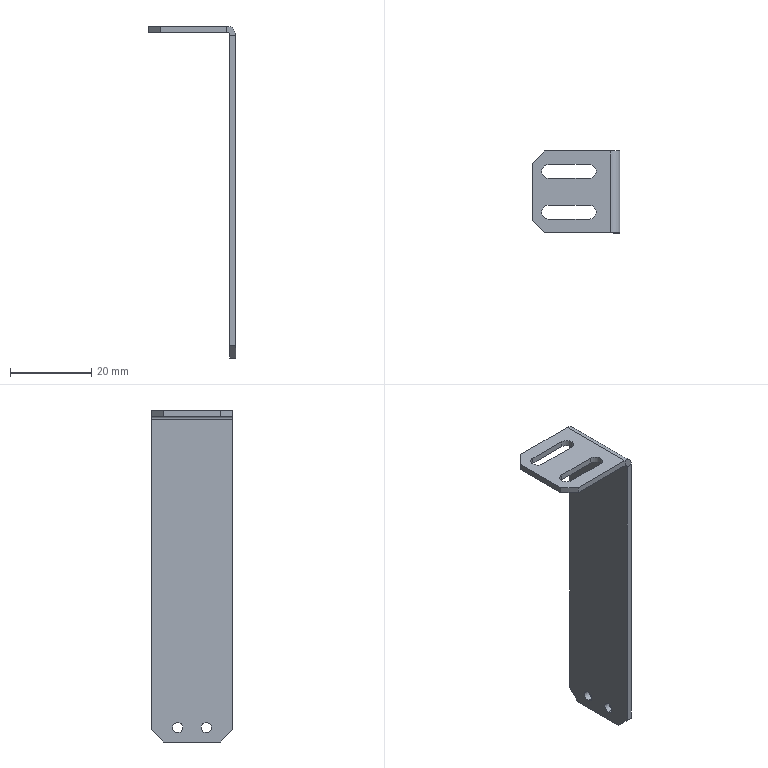Part | SolidWorks | features HoleWzd 2, Chamfer 1, FlatPattern 1, SMBaseFlange 1, SheetMetal 1 | 1 solid | 32 faces | box 21.5 x 20 x 81.5 mm | volume 2855 mm3 | plane 20 | cylinder 12 | commonest cylinder face diameters 3.4 x6 2.5 x4 1.473 x1 4.473 x1
STEP:
#1=CARTESIAN_POINT('',(-17.7,15.,1.5));
#2=VERTEX_POINT('',#1);
#3=CARTESIAN_POINT('',(-16.,16.7,1.5));
#4=VERTEX_POINT('',#3);
#5=CARTESIAN_POINT('',(-16.,15.,1.5));
#6=DIRECTION('',(0.,0.,-1.));
#7=DIRECTION('',(-1.,0.,0.));
#8=AXIS2_PLACEMENT_3D('',#5,#6,#7);
#9=CIRCLE('',#8,1.7);
#10=EDGE_CURVE('',#2,#4,#9,.T.);
#11=ORIENTED_EDGE('',*,*,#10,.F.);
#12=CARTESIAN_POINT('',(-17.7,15.,0.));
#13=VERTEX_POINT('',#12);
#14=CARTESIAN_POINT('',(-17.7,15.,0.));
#15=DIRECTION('',(0.,0.,-1.));
#16=VECTOR('',#15,1000.);
#17=LINE('',#14,#16);
#18=EDGE_CURVE('',#2,#13,#17,.T.);
#19=ORIENTED_EDGE('',*,*,#18,.T.);
#20=CARTESIAN_POINT('',(-16.,16.7,0.));
#21=VERTEX_POINT('',#20);
#22=CARTESIAN_POINT('',(-16.,15.,0.));
#23=DIRECTION('',(0.,0.,-1.));
#24=DIRECTION('',(-1.,0.,0.));
#25=AXIS2_PLACEMENT_3D('',#22,#23,#24);
#26=CIRCLE('',#25,1.7);
#27=EDGE_CURVE('',#13,#21,#26,.T.);
#28=ORIENTED_EDGE('',*,*,#27,.T.);
#29=CARTESIAN_POINT('',(-16.,16.7,0.));
#30=DIRECTION('',(0.,0.,-1.));
#31=VECTOR('',#30,1000.);
#32=LINE('',#29,#31);
#33=EDGE_CURVE('',#4,#21,#32,.T.);
#34=ORIENTED_EDGE('',*,*,#33,.F.);
#35=EDGE_LOOP('',(#11,#19,#28,#34));
#36=FACE_OUTER_BOUND('',#35,.T.);
#37=CARTESIAN_POINT('',(-16.,15.,0.));
#38=DIRECTION('',(0.,0.,-1.));
#39=DIRECTION('',(-1.,0.,0.));
#40=AXIS2_PLACEMENT_3D('',#37,#38,#39);
#41=CYLINDRICAL_SURFACE('',#40,1.7);
#42=ADVANCED_FACE('',(#36),#41,.F.);
#43=CARTESIAN_POINT('',(-17.7,5.,1.5));
#44=VERTEX_POINT('',#43);
#45=CARTESIAN_POINT('',(-16.,6.7,1.5));
#46=VERTEX_POINT('',#45);
#47=CARTESIAN_POINT('',(-16.,5.,1.5));
#48=DIRECTION('',(0.,0.,-1.));
#49=DIRECTION('',(-1.,0.,0.));
#50=AXIS2_PLACEMENT_3D('',#47,#48,#49);
#51=CIRCLE('',#50,1.7);
#52=EDGE_CURVE('',#44,#46,#51,.T.);
#53=ORIENTED_EDGE('',*,*,#52,.F.);
#54=CARTESIAN_POINT('',(-17.7,5.,0.));
#55=VERTEX_POINT('',#54);
#56=CARTESIAN_POINT('',(-17.7,5.,0.));
#57=DIRECTION('',(0.,0.,-1.));
#58=VECTOR('',#57,1000.);
#59=LINE('',#56,#58);
#60=EDGE_CURVE('',#44,#55,#59,.T.);
#61=ORIENTED_EDGE('',*,*,#60,.T.);
#62=CARTESIAN_POINT('',(-16.,6.7,0.));
#63=VERTEX_POINT('',#62);
#64=CARTESIAN_POINT('',(-16.,5.,0.));
#65=DIRECTION('',(0.,0.,-1.));
#66=DIRECTION('',(-1.,0.,0.));
#67=AXIS2_PLACEMENT_3D('',#64,#65,#66);
#68=CIRCLE('',#67,1.7);
#69=EDGE_CURVE('',#55,#63,#68,.T.);
#70=ORIENTED_EDGE('',*,*,#69,.T.);
#71=CARTESIAN_POINT('',(-16.,6.7,0.));
#72=DIRECTION('',(0.,0.,-1.));
#73=VECTOR('',#72,1000.);
#74=LINE('',#71,#73);
#75=EDGE_CURVE('',#46,#63,#74,.T.);
#76=ORIENTED_EDGE('',*,*,#75,.F.);
#77=EDGE_LOOP('',(#53,#61,#70,#76));
#78=FACE_OUTER_BOUND('',#77,.T.);
#79=CARTESIAN_POINT('',(-16.,5.,0.));
#80=DIRECTION('',(0.,0.,-1.));
#81=DIRECTION('',(-1.,0.,0.));
#82=AXIS2_PLACEMENT_3D('',#79,#80,#81);
#83=CYLINDRICAL_SURFACE('',#82,1.7);
#84=ADVANCED_FACE('',(#78),#83,.F.);
#85=CARTESIAN_POINT('',(0.,13.5,-77.75));
#86=VERTEX_POINT('',#85);
#87=CARTESIAN_POINT('',(0.,13.5,-75.25));
#88=VERTEX_POINT('',#87);
#89=CARTESIAN_POINT('',(0.,13.5,-76.5));
#90=DIRECTION('',(-1.,0.,0.));
#91=DIRECTION('',(0.,0.,1.));
#92=AXIS2_PLACEMENT_3D('',#89,#90,#91);
#93=CIRCLE('',#92,1.25);
#94=EDGE_CURVE('',#86,#88,#93,.T.);
#95=ORIENTED_EDGE('',*,*,#94,.T.);
#96=CARTESIAN_POINT('',(1.5,13.5,-75.25));
#97=VERTEX_POINT('',#96);
#98=CARTESIAN_POINT('',(1.5,13.5,-75.25));
#99=DIRECTION('',(1.,0.,0.));
#100=VECTOR('',#99,1000.);
#101=LINE('',#98,#100);
#102=EDGE_CURVE('',#88,#97,#101,.T.);
#103=ORIENTED_EDGE('',*,*,#102,.T.);
#104=CARTESIAN_POINT('',(1.5,13.5,-77.75));
#105=VERTEX_POINT('',#104);
#106=CARTESIAN_POINT('',(1.5,13.5,-76.5));
#107=DIRECTION('',(1.,0.,0.));
#108=DIRECTION('',(0.,0.,-1.));
#109=AXIS2_PLACEMENT_3D('',#106,#107,#108);
#110=CIRCLE('',#109,1.25);
#111=EDGE_CURVE('',#97,#105,#110,.T.);
#112=ORIENTED_EDGE('',*,*,#111,.T.);
#113=CARTESIAN_POINT('',(1.5,13.5,-77.75));
#114=DIRECTION('',(1.,0.,0.));
#115=VECTOR('',#114,1000.);
#116=LINE('',#113,#115);
#117=EDGE_CURVE('',#86,#105,#116,.T.);
#118=ORIENTED_EDGE('',*,*,#117,.F.);
#119=EDGE_LOOP('',(#95,#103,#112,#118));
#120=FACE_OUTER_BOUND('',#119,.T.);
#121=CARTESIAN_POINT('',(1.5,13.5,-76.5));
#122=DIRECTION('',(1.,0.,0.));
#123=DIRECTION('',(0.,0.,-1.));
#124=AXIS2_PLACEMENT_3D('',#121,#122,#123);
#125=CYLINDRICAL_SURFACE('',#124,1.25);
#126=ADVANCED_FACE('',(#120),#125,.F.);
#127=CARTESIAN_POINT('',(0.,6.5,-77.75));
#128=VERTEX_POINT('',#127);
#129=CARTESIAN_POINT('',(0.,6.5,-75.25));
#130=VERTEX_POINT('',#129);
#131=CARTESIAN_POINT('',(0.,6.5,-76.5));
#132=DIRECTION('',(-1.,0.,0.));
#133=DIRECTION('',(0.,0.,1.));
#134=AXIS2_PLACEMENT_3D('',#131,#132,#133);
#135=CIRCLE('',#134,1.25);
#136=EDGE_CURVE('',#128,#130,#135,.T.);
#137=ORIENTED_EDGE('',*,*,#136,.T.);
#138=CARTESIAN_POINT('',(1.5,6.5,-75.25));
#139=VERTEX_POINT('',#138);
#140=CARTESIAN_POINT('',(1.5,6.5,-75.25));
#141=DIRECTION('',(1.,0.,0.));
#142=VECTOR('',#141,1000.);
#143=LINE('',#140,#142);
#144=EDGE_CURVE('',#130,#139,#143,.T.);
#145=ORIENTED_EDGE('',*,*,#144,.T.);
#146=CARTESIAN_POINT('',(1.5,6.5,-77.75));
#147=VERTEX_POINT('',#146);
#148=CARTESIAN_POINT('',(1.5,6.5,-76.5));
#149=DIRECTION('',(1.,0.,0.));
#150=DIRECTION('',(0.,0.,-1.));
#151=AXIS2_PLACEMENT_3D('',#148,#149,#150);
#152=CIRCLE('',#151,1.25);
#153=EDGE_CURVE('',#139,#147,#152,.T.);
#154=ORIENTED_EDGE('',*,*,#153,.T.);
#155=CARTESIAN_POINT('',(1.5,6.5,-77.75));
#156=DIRECTION('',(1.,0.,0.));
#157=VECTOR('',#156,1000.);
#158=LINE('',#155,#157);
#159=EDGE_CURVE('',#128,#147,#158,.T.);
#160=ORIENTED_EDGE('',*,*,#159,.F.);
#161=EDGE_LOOP('',(#137,#145,#154,#160));
#162=FACE_OUTER_BOUND('',#161,.T.);
#163=CARTESIAN_POINT('',(1.5,6.5,-76.5));
#164=DIRECTION('',(1.,0.,0.));
#165=DIRECTION('',(0.,0.,-1.));
#166=AXIS2_PLACEMENT_3D('',#163,#164,#165);
#167=CYLINDRICAL_SURFACE('',#166,1.25);
#168=ADVANCED_FACE('',(#162),#167,.F.);
#169=CARTESIAN_POINT('',(0.,20.,-0.7366));
#170=VERTEX_POINT('',#169);
#171=CARTESIAN_POINT('',(1.5,20.,-0.7366));
#172=VERTEX_POINT('',#171);
#173=CARTESIAN_POINT('',(0.,20.,-0.7366));
#174=DIRECTION('',(1.,0.,0.));
#175=VECTOR('',#174,1000.);
#176=LINE('',#173,#175);
#177=EDGE_CURVE('',#170,#172,#176,.T.);
#178=ORIENTED_EDGE('',*,*,#177,.F.);
#179=CARTESIAN_POINT('',(-0.7366,20.,0.));
#180=VERTEX_POINT('',#179);
#181=CARTESIAN_POINT('',(-0.7366,20.,-0.7366));
#182=DIRECTION('',(0.,1.,0.));
#183=DIRECTION('',(0.,0.,-1.));
#184=AXIS2_PLACEMENT_3D('',#181,#182,#183);
#185=CIRCLE('',#184,0.7366);
#186=EDGE_CURVE('',#180,#170,#185,.T.);
#187=ORIENTED_EDGE('',*,*,#186,.F.);
#188=CARTESIAN_POINT('',(-0.7366,20.,1.5));
#189=VERTEX_POINT('',#188);
#190=CARTESIAN_POINT('',(-0.7366,20.,1.5));
#191=DIRECTION('',(0.,0.,-1.));
#192=VECTOR('',#191,1000.);
#193=LINE('',#190,#192);
#194=EDGE_CURVE('',#189,#180,#193,.T.);
#195=ORIENTED_EDGE('',*,*,#194,.F.);
#196=CARTESIAN_POINT('',(-0.7366,20.,-0.7366));
#197=DIRECTION('',(0.,1.,0.));
#198=DIRECTION('',(1.,0.,0.));
#199=AXIS2_PLACEMENT_3D('',#196,#197,#198);
#200=CIRCLE('',#199,2.237);
#201=EDGE_CURVE('',#189,#172,#200,.T.);
#202=ORIENTED_EDGE('',*,*,#201,.T.);
#203=EDGE_LOOP('',(#178,#187,#195,#202));
#204=FACE_OUTER_BOUND('',#203,.T.);
#205=CARTESIAN_POINT('',(0.,20.,-0.7366));
#206=DIRECTION('',(0.,1.,0.));
#207=DIRECTION('',(0.,0.,1.));
#208=AXIS2_PLACEMENT_3D('',#205,#206,#207);
#209=PLANE('',#208);
#210=ADVANCED_FACE('',(#204),#209,.T.);
#211=CARTESIAN_POINT('',(1.5,20.,-77.));
#212=VERTEX_POINT('',#211);
#213=CARTESIAN_POINT('',(1.5,20.,0.));
#214=DIRECTION('',(0.,0.,-1.));
#215=VECTOR('',#214,1000.);
#216=LINE('',#213,#215);
#217=EDGE_CURVE('',#172,#212,#216,.T.);
#218=ORIENTED_EDGE('',*,*,#217,.T.);
#219=CARTESIAN_POINT('',(0.,20.,-77.));
#220=VERTEX_POINT('',#219);
#221=CARTESIAN_POINT('',(-0.7366,20.,-77.));
#222=DIRECTION('',(-1.,0.,0.));
#223=VECTOR('',#222,1000.);
#224=LINE('',#221,#223);
#225=EDGE_CURVE('',#212,#220,#224,.T.);
#226=ORIENTED_EDGE('',*,*,#225,.T.);
#227=CARTESIAN_POINT('',(0.,20.,0.));
#228=DIRECTION('',(0.,0.,-1.));
#229=VECTOR('',#228,1000.);
#230=LINE('',#227,#229);
#231=EDGE_CURVE('',#170,#220,#230,.T.);
#232=ORIENTED_EDGE('',*,*,#231,.F.);
#233=ORIENTED_EDGE('',*,*,#177,.T.);
#234=EDGE_LOOP('',(#218,#226,#232,#233));
#235=FACE_OUTER_BOUND('',#234,.T.);
#236=CARTESIAN_POINT('',(-0.7366,20.,1.5));
#237=DIRECTION('',(0.,1.,0.));
#238=DIRECTION('',(0.,0.,1.));
#239=AXIS2_PLACEMENT_3D('',#236,#237,#238);
#240=PLANE('',#239);
#241=ADVANCED_FACE('',(#235),#240,.T.);
#242=CARTESIAN_POINT('',(-0.7366,0.,0.));
#243=VERTEX_POINT('',#242);
#244=CARTESIAN_POINT('',(-0.7366,0.,1.5));
#245=VERTEX_POINT('',#244);
#246=CARTESIAN_POINT('',(-0.7366,0.,0.));
#247=DIRECTION('',(0.,0.,1.));
#248=VECTOR('',#247,1000.);
#249=LINE('',#246,#248);
#250=EDGE_CURVE('',#243,#245,#249,.T.);
#251=ORIENTED_EDGE('',*,*,#250,.F.);
#252=CARTESIAN_POINT('',(0.,0.,-0.7366));
#253=VERTEX_POINT('',#252);
#254=CARTESIAN_POINT('',(-0.7366,0.,-0.7366));
#255=DIRECTION('',(0.,1.,0.));
#256=DIRECTION('',(0.,0.,-1.));
#257=AXIS2_PLACEMENT_3D('',#254,#255,#256);
#258=CIRCLE('',#257,0.7366);
#259=EDGE_CURVE('',#243,#253,#258,.T.);
#260=ORIENTED_EDGE('',*,*,#259,.T.);
#261=CARTESIAN_POINT('',(1.5,0.,-0.7366));
#262=VERTEX_POINT('',#261);
#263=CARTESIAN_POINT('',(1.5,0.,-0.7366));
#264=DIRECTION('',(-1.,0.,0.));
#265=VECTOR('',#264,1000.);
#266=LINE('',#263,#265);
#267=EDGE_CURVE('',#262,#253,#266,.T.);
#268=ORIENTED_EDGE('',*,*,#267,.F.);
#269=CARTESIAN_POINT('',(-0.7366,0.,-0.7366));
#270=DIRECTION('',(0.,1.,0.));
#271=DIRECTION('',(1.,0.,0.));
#272=AXIS2_PLACEMENT_3D('',#269,#270,#271);
#273=CIRCLE('',#272,2.237);
#274=EDGE_CURVE('',#245,#262,#273,.T.);
#275=ORIENTED_EDGE('',*,*,#274,.F.);
#276=EDGE_LOOP('',(#251,#260,#268,#275));
#277=FACE_OUTER_BOUND('',#276,.T.);
#278=CARTESIAN_POINT('',(-0.7366,0.,0.));
#279=DIRECTION('',(0.,-1.,0.));
#280=DIRECTION('',(0.,0.,-1.));
#281=AXIS2_PLACEMENT_3D('',#278,#279,#280);
#282=PLANE('',#281);
#283=ADVANCED_FACE('',(#277),#282,.T.);
#284=CARTESIAN_POINT('',(-17.,0.,1.5));
#285=VERTEX_POINT('',#284);
#286=CARTESIAN_POINT('',(-20.,0.,1.5));
#287=DIRECTION('',(1.,0.,0.));
#288=VECTOR('',#287,1000.);
#289=LINE('',#286,#288);
#290=EDGE_CURVE('',#285,#245,#289,.T.);
#291=ORIENTED_EDGE('',*,*,#290,.F.);
#292=CARTESIAN_POINT('',(-17.,0.,0.));
#293=VERTEX_POINT('',#292);
#294=CARTESIAN_POINT('',(-17.,0.,-0.7366));
#295=DIRECTION('',(0.,0.,-1.));
#296=VECTOR('',#295,1000.);
#297=LINE('',#294,#296);
#298=EDGE_CURVE('',#285,#293,#297,.T.);
#299=ORIENTED_EDGE('',*,*,#298,.T.);
#300=CARTESIAN_POINT('',(-20.,0.,0.));
#301=DIRECTION('',(1.,0.,0.));
#302=VECTOR('',#301,1000.);
#303=LINE('',#300,#302);
#304=EDGE_CURVE('',#293,#243,#303,.T.);
#305=ORIENTED_EDGE('',*,*,#304,.T.);
#306=ORIENTED_EDGE('',*,*,#250,.T.);
#307=EDGE_LOOP('',(#291,#299,#305,#306));
#308=FACE_OUTER_BOUND('',#307,.T.);
#309=CARTESIAN_POINT('',(1.5,0.,-0.7366));
#310=DIRECTION('',(0.,-1.,0.));
#311=DIRECTION('',(0.,0.,-1.));
#312=AXIS2_PLACEMENT_3D('',#309,#310,#311);
#313=PLANE('',#312);
#314=ADVANCED_FACE('',(#308),#313,.T.);
#315=CARTESIAN_POINT('',(1.5,13.5,-76.5));
#316=DIRECTION('',(1.,0.,0.));
#317=DIRECTION('',(0.,0.,-1.));
#318=AXIS2_PLACEMENT_3D('',#315,#316,#317);
#319=CIRCLE('',#318,1.25);
#320=EDGE_CURVE('',#105,#97,#319,.T.);
#321=ORIENTED_EDGE('',*,*,#320,.F.);
#322=ORIENTED_EDGE('',*,*,#111,.F.);
#323=EDGE_LOOP('',(#321,#322));
#324=FACE_BOUND('',#323,.T.);
#325=CARTESIAN_POINT('',(1.5,6.5,-76.5));
#326=DIRECTION('',(1.,0.,0.));
#327=DIRECTION('',(0.,0.,-1.));
#328=AXIS2_PLACEMENT_3D('',#325,#326,#327);
#329=CIRCLE('',#328,1.25);
#330=EDGE_CURVE('',#147,#139,#329,.T.);
#331=ORIENTED_EDGE('',*,*,#330,.F.);
#332=ORIENTED_EDGE('',*,*,#153,.F.);
#333=EDGE_LOOP('',(#331,#332));
#334=FACE_BOUND('',#333,.T.);
#335=CARTESIAN_POINT('',(1.5,0.,-77.));
#336=VERTEX_POINT('',#335);
#337=CARTESIAN_POINT('',(1.5,0.,0.));
#338=DIRECTION('',(0.,0.,-1.));
#339=VECTOR('',#338,1000.);
#340=LINE('',#337,#339);
#341=EDGE_CURVE('',#262,#336,#340,.T.);
#342=ORIENTED_EDGE('',*,*,#341,.T.);
#343=CARTESIAN_POINT('',(1.5,3.,-80.));
#344=VERTEX_POINT('',#343);
#345=CARTESIAN_POINT('',(1.5,0.,-77.));
#346=DIRECTION('',(0.,0.7071,-0.7071));
#347=VECTOR('',#346,1000.);
#348=LINE('',#345,#347);
#349=EDGE_CURVE('',#336,#344,#348,.T.);
#350=ORIENTED_EDGE('',*,*,#349,.T.);
#351=CARTESIAN_POINT('',(1.5,17.,-80.));
#352=VERTEX_POINT('',#351);
#353=CARTESIAN_POINT('',(1.5,20.,-80.));
#354=DIRECTION('',(0.,-1.,0.));
#355=VECTOR('',#354,1000.);
#356=LINE('',#353,#355);
#357=EDGE_CURVE('',#352,#344,#356,.T.);
#358=ORIENTED_EDGE('',*,*,#357,.F.);
#359=CARTESIAN_POINT('',(1.5,17.,-80.));
#360=DIRECTION('',(0.,0.7071,0.7071));
#361=VECTOR('',#360,1000.);
#362=LINE('',#359,#361);
#363=EDGE_CURVE('',#352,#212,#362,.T.);
#364=ORIENTED_EDGE('',*,*,#363,.T.);
#365=ORIENTED_EDGE('',*,*,#217,.F.);
#366=CARTESIAN_POINT('',(1.5,20.,-0.7366));
#367=DIRECTION('',(0.,-1.,0.));
#368=VECTOR('',#367,1000.);
#369=LINE('',#366,#368);
#370=EDGE_CURVE('',#172,#262,#369,.T.);
#371=ORIENTED_EDGE('',*,*,#370,.T.);
#372=EDGE_LOOP('',(#342,#350,#358,#364,#365,#371));
#373=FACE_OUTER_BOUND('',#372,.T.);
#374=CARTESIAN_POINT('',(1.5,20.,0.));
#375=DIRECTION('',(-1.,0.,0.));
#376=DIRECTION('',(0.,0.,1.));
#377=AXIS2_PLACEMENT_3D('',#374,#375,#376);
#378=PLANE('',#377);
#379=ADVANCED_FACE('',(#324,#334,#373),#378,.F.);
#380=ORIENTED_EDGE('',*,*,#357,.T.);
#381=CARTESIAN_POINT('',(0.,3.,-80.));
#382=VERTEX_POINT('',#381);
#383=CARTESIAN_POINT('',(0.,3.,-80.));
#384=DIRECTION('',(-1.,0.,0.));
#385=VECTOR('',#384,1000.);
#386=LINE('',#383,#385);
#387=EDGE_CURVE('',#344,#382,#386,.T.);
#388=ORIENTED_EDGE('',*,*,#387,.T.);
#389=CARTESIAN_POINT('',(0.,17.,-80.));
#390=VERTEX_POINT('',#389);
#391=CARTESIAN_POINT('',(0.,20.,-80.));
#392=DIRECTION('',(0.,-1.,0.));
#393=VECTOR('',#392,1000.);
#394=LINE('',#391,#393);
#395=EDGE_CURVE('',#390,#382,#394,.T.);
#396=ORIENTED_EDGE('',*,*,#395,.F.);
#397=CARTESIAN_POINT('',(0.,17.,-80.));
#398=DIRECTION('',(1.,0.,0.));
#399=VECTOR('',#398,1000.);
#400=LINE('',#397,#399);
#401=EDGE_CURVE('',#390,#352,#400,.T.);
#402=ORIENTED_EDGE('',*,*,#401,.T.);
#403=EDGE_LOOP('',(#380,#388,#396,#402));
#404=FACE_OUTER_BOUND('',#403,.T.);
#405=CARTESIAN_POINT('',(0.,20.,-80.));
#406=DIRECTION('',(0.,0.,-1.));
#407=DIRECTION('',(-1.,0.,0.));
#408=AXIS2_PLACEMENT_3D('',#405,#406,#407);
#409=PLANE('',#408);
#410=ADVANCED_FACE('',(#404),#409,.T.);
#411=ORIENTED_EDGE('',*,*,#94,.F.);
#412=CARTESIAN_POINT('',(0.,13.5,-76.5));
#413=DIRECTION('',(-1.,0.,0.));
#414=DIRECTION('',(0.,0.,1.));
#415=AXIS2_PLACEMENT_3D('',#412,#413,#414);
#416=CIRCLE('',#415,1.25);
#417=EDGE_CURVE('',#88,#86,#416,.T.);
#418=ORIENTED_EDGE('',*,*,#417,.F.);
#419=EDGE_LOOP('',(#411,#418));
#420=FACE_BOUND('',#419,.T.);
#421=ORIENTED_EDGE('',*,*,#136,.F.);
#422=CARTESIAN_POINT('',(0.,6.5,-76.5));
#423=DIRECTION('',(-1.,0.,0.));
#424=DIRECTION('',(0.,0.,1.));
#425=AXIS2_PLACEMENT_3D('',#422,#423,#424);
#426=CIRCLE('',#425,1.25);
#427=EDGE_CURVE('',#130,#128,#426,.T.);
#428=ORIENTED_EDGE('',*,*,#427,.F.);
#429=EDGE_LOOP('',(#421,#428));
#430=FACE_BOUND('',#429,.T.);
#431=ORIENTED_EDGE('',*,*,#395,.T.);
#432=CARTESIAN_POINT('',(0.,0.,-77.));
#433=VERTEX_POINT('',#432);
#434=CARTESIAN_POINT('',(0.,-28.5,-48.5));
#435=DIRECTION('',(0.,-0.7071,0.7071));
#436=VECTOR('',#435,1000.);
#437=LINE('',#434,#436);
#438=EDGE_CURVE('',#382,#433,#437,.T.);
#439=ORIENTED_EDGE('',*,*,#438,.T.);
#440=CARTESIAN_POINT('',(0.,0.,0.));
#441=DIRECTION('',(0.,0.,-1.));
#442=VECTOR('',#441,1000.);
#443=LINE('',#440,#442);
#444=EDGE_CURVE('',#253,#433,#443,.T.);
#445=ORIENTED_EDGE('',*,*,#444,.F.);
#446=CARTESIAN_POINT('',(0.,20.,-0.7366));
#447=DIRECTION('',(0.,-1.,0.));
#448=VECTOR('',#447,1000.);
#449=LINE('',#446,#448);
#450=EDGE_CURVE('',#170,#253,#449,.T.);
#451=ORIENTED_EDGE('',*,*,#450,.F.);
#452=ORIENTED_EDGE('',*,*,#231,.T.);
#453=CARTESIAN_POINT('',(0.,58.5,-38.5));
#454=DIRECTION('',(0.,-0.7071,-0.7071));
#455=VECTOR('',#454,1000.);
#456=LINE('',#453,#455);
#457=EDGE_CURVE('',#220,#390,#456,.T.);
#458=ORIENTED_EDGE('',*,*,#457,.T.);
#459=EDGE_LOOP('',(#431,#439,#445,#451,#452,#458));
#460=FACE_OUTER_BOUND('',#459,.T.);
#461=CARTESIAN_POINT('',(0.,20.,0.));
#462=DIRECTION('',(-1.,0.,0.));
#463=DIRECTION('',(0.,0.,1.));
#464=AXIS2_PLACEMENT_3D('',#461,#462,#463);
#465=PLANE('',#464);
#466=ADVANCED_FACE('',(#420,#430,#460),#465,.T.);
#467=ORIENTED_EDGE('',*,*,#259,.F.);
#468=CARTESIAN_POINT('',(-0.7366,20.,0.));
#469=DIRECTION('',(0.,-1.,0.));
#470=VECTOR('',#469,1000.);
#471=LINE('',#468,#470);
#472=EDGE_CURVE('',#180,#243,#471,.T.);
#473=ORIENTED_EDGE('',*,*,#472,.F.);
#474=ORIENTED_EDGE('',*,*,#186,.T.);
#475=ORIENTED_EDGE('',*,*,#450,.T.);
#476=EDGE_LOOP('',(#467,#473,#474,#475));
#477=FACE_OUTER_BOUND('',#476,.T.);
#478=CARTESIAN_POINT('',(-0.7366,20.,-0.7366));
#479=DIRECTION('',(0.,-1.,0.));
#480=DIRECTION('',(0.,0.,-1.));
#481=AXIS2_PLACEMENT_3D('',#478,#479,#480);
#482=CYLINDRICAL_SURFACE('',#481,0.7366);
#483=ADVANCED_FACE('',(#477),#482,.F.);
#484=CARTESIAN_POINT('',(-6.,16.7,0.));
#485=VERTEX_POINT('',#484);
#486=CARTESIAN_POINT('',(-6.,13.3,0.));
#487=VERTEX_POINT('',#486);
#488=CARTESIAN_POINT('',(-6.,15.,0.));
#489=DIRECTION('',(0.,0.,-1.));
#490=DIRECTION('',(-1.,0.,0.));
#491=AXIS2_PLACEMENT_3D('',#488,#489,#490);
#492=CIRCLE('',#491,1.7);
#493=EDGE_CURVE('',#485,#487,#492,.T.);
#494=ORIENTED_EDGE('',*,*,#493,.F.);
#495=CARTESIAN_POINT('',(-16.,16.7,0.));
#496=DIRECTION('',(1.,0.,0.));
#497=VECTOR('',#496,1000.);
#498=LINE('',#495,#497);
#499=EDGE_CURVE('',#21,#485,#498,.T.);
#500=ORIENTED_EDGE('',*,*,#499,.F.);
#501=ORIENTED_EDGE('',*,*,#27,.F.);
#502=CARTESIAN_POINT('',(-16.,13.3,0.));
#503=VERTEX_POINT('',#502);
#504=CARTESIAN_POINT('',(-16.,15.,0.));
#505=DIRECTION('',(0.,0.,-1.));
#506=DIRECTION('',(-1.,0.,0.));
#507=AXIS2_PLACEMENT_3D('',#504,#505,#506);
#508=CIRCLE('',#507,1.7);
#509=EDGE_CURVE('',#503,#13,#508,.T.);
#510=ORIENTED_EDGE('',*,*,#509,.F.);
#511=CARTESIAN_POINT('',(-16.,13.3,0.));
#512=DIRECTION('',(1.,0.,0.));
#513=VECTOR('',#512,1000.);
#514=LINE('',#511,#513);
#515=EDGE_CURVE('',#503,#487,#514,.T.);
#516=ORIENTED_EDGE('',*,*,#515,.T.);
#517=EDGE_LOOP('',(#494,#500,#501,#510,#516));
#518=FACE_BOUND('',#517,.T.);
#519=CARTESIAN_POINT('',(-6.,6.7,0.));
#520=VERTEX_POINT('',#519);
#521=CARTESIAN_POINT('',(-16.,6.7,0.));
#522=DIRECTION('',(1.,0.,0.));
#523=VECTOR('',#522,1000.);
#524=LINE('',#521,#523);
#525=EDGE_CURVE('',#63,#520,#524,.T.);
#526=ORIENTED_EDGE('',*,*,#525,.F.);
#527=ORIENTED_EDGE('',*,*,#69,.F.);
#528=CARTESIAN_POINT('',(-16.,3.3,0.));
#529=VERTEX_POINT('',#528);
#530=CARTESIAN_POINT('',(-16.,5.,0.));
#531=DIRECTION('',(0.,0.,-1.));
#532=DIRECTION('',(-1.,0.,0.));
#533=AXIS2_PLACEMENT_3D('',#530,#531,#532);
#534=CIRCLE('',#533,1.7);
#535=EDGE_CURVE('',#529,#55,#534,.T.);
#536=ORIENTED_EDGE('',*,*,#535,.F.);
#537=CARTESIAN_POINT('',(-6.,3.3,0.));
#538=VERTEX_POINT('',#537);
#539=CARTESIAN_POINT('',(-16.,3.3,0.));
#540=DIRECTION('',(1.,0.,0.));
#541=VECTOR('',#540,1000.);
#542=LINE('',#539,#541);
#543=EDGE_CURVE('',#529,#538,#542,.T.);
#544=ORIENTED_EDGE('',*,*,#543,.T.);
#545=CARTESIAN_POINT('',(-6.,5.,0.));
#546=DIRECTION('',(0.,0.,-1.));
#547=DIRECTION('',(-1.,0.,0.));
#548=AXIS2_PLACEMENT_3D('',#545,#546,#547);
#549=CIRCLE('',#548,1.7);
#550=EDGE_CURVE('',#520,#538,#549,.T.);
#551=ORIENTED_EDGE('',*,*,#550,.F.);
#552=EDGE_LOOP('',(#526,#527,#536,#544,#551));
#553=FACE_BOUND('',#552,.T.);
#554=CARTESIAN_POINT('',(-20.,17.,0.));
#555=VERTEX_POINT('',#554);
#556=CARTESIAN_POINT('',(-20.,3.,0.));
#557=VERTEX_POINT('',#556);
#558=CARTESIAN_POINT('',(-20.,20.,0.));
#559=DIRECTION('',(0.,-1.,0.));
#560=VECTOR('',#559,1000.);
#561=LINE('',#558,#560);
#562=EDGE_CURVE('',#555,#557,#561,.T.);
#563=ORIENTED_EDGE('',*,*,#562,.F.);
#564=CARTESIAN_POINT('',(-17.,20.,0.));
#565=VERTEX_POINT('',#564);
#566=CARTESIAN_POINT('',(-18.5,18.5,0.));
#567=DIRECTION('',(0.7071,0.7071,0.));
#568=VECTOR('',#567,1000.);
#569=LINE('',#566,#568);
#570=EDGE_CURVE('',#555,#565,#569,.T.);
#571=ORIENTED_EDGE('',*,*,#570,.T.);
#572=CARTESIAN_POINT('',(-20.,20.,0.));
#573=DIRECTION('',(1.,0.,0.));
#574=VECTOR('',#573,1000.);
#575=LINE('',#572,#574);
#576=EDGE_CURVE('',#565,#180,#575,.T.);
#577=ORIENTED_EDGE('',*,*,#576,.T.);
#578=ORIENTED_EDGE('',*,*,#472,.T.);
#579=ORIENTED_EDGE('',*,*,#304,.F.);
#580=CARTESIAN_POINT('',(-28.5,11.5,0.));
#581=DIRECTION('',(-0.7071,0.7071,0.));
#582=VECTOR('',#581,1000.);
#583=LINE('',#580,#582);
#584=EDGE_CURVE('',#293,#557,#583,.T.);
#585=ORIENTED_EDGE('',*,*,#584,.T.);
#586=EDGE_LOOP('',(#563,#571,#577,#578,#579,#585));
#587=FACE_OUTER_BOUND('',#586,.T.);
#588=CARTESIAN_POINT('',(-20.,20.,0.));
#589=DIRECTION('',(0.,0.,-1.));
#590=DIRECTION('',(-1.,0.,0.));
#591=AXIS2_PLACEMENT_3D('',#588,#589,#590);
#592=PLANE('',#591);
#593=ADVANCED_FACE('',(#518,#553,#587),#592,.T.);
#594=CARTESIAN_POINT('',(-20.,17.,1.5));
#595=VERTEX_POINT('',#594);
#596=CARTESIAN_POINT('',(-20.,3.,1.5));
#597=VERTEX_POINT('',#596);
#598=CARTESIAN_POINT('',(-20.,20.,1.5));
#599=DIRECTION('',(0.,-1.,0.));
#600=VECTOR('',#599,1000.);
#601=LINE('',#598,#600);
#602=EDGE_CURVE('',#595,#597,#601,.T.);
#603=ORIENTED_EDGE('',*,*,#602,.F.);
#604=CARTESIAN_POINT('',(-20.,17.,0.));
#605=DIRECTION('',(0.,0.,-1.));
#606=VECTOR('',#605,1000.);
#607=LINE('',#604,#606);
#608=EDGE_CURVE('',#595,#555,#607,.T.);
#609=ORIENTED_EDGE('',*,*,#608,.T.);
#610=ORIENTED_EDGE('',*,*,#562,.T.);
#611=CARTESIAN_POINT('',(-20.,3.,1.5));
#612=DIRECTION('',(0.,0.,1.));
#613=VECTOR('',#612,1000.);
#614=LINE('',#611,#613);
#615=EDGE_CURVE('',#557,#597,#614,.T.);
#616=ORIENTED_EDGE('',*,*,#615,.T.);
#617=EDGE_LOOP('',(#603,#609,#610,#616));
#618=FACE_OUTER_BOUND('',#617,.T.);
#619=CARTESIAN_POINT('',(-20.,20.,1.5));
#620=DIRECTION('',(-1.,0.,0.));
#621=DIRECTION('',(0.,0.,1.));
#622=AXIS2_PLACEMENT_3D('',#619,#620,#621);
#623=PLANE('',#622);
#624=ADVANCED_FACE('',(#618),#623,.T.);
#625=CARTESIAN_POINT('',(-6.,16.7,1.5));
#626=VERTEX_POINT('',#625);
#627=CARTESIAN_POINT('',(-6.,13.3,1.5));
#628=VERTEX_POINT('',#627);
#629=CARTESIAN_POINT('',(-6.,15.,1.5));
#630=DIRECTION('',(0.,0.,-1.));
#631=DIRECTION('',(-1.,0.,0.));
#632=AXIS2_PLACEMENT_3D('',#629,#630,#631);
#633=CIRCLE('',#632,1.7);
#634=EDGE_CURVE('',#626,#628,#633,.T.);
#635=ORIENTED_EDGE('',*,*,#634,.T.);
#636=CARTESIAN_POINT('',(-16.,13.3,1.5));
#637=VERTEX_POINT('',#636);
#638=CARTESIAN_POINT('',(-20.,13.3,1.5));
#639=DIRECTION('',(-1.,0.,0.));
#640=VECTOR('',#639,1000.);
#641=LINE('',#638,#640);
#642=EDGE_CURVE('',#628,#637,#641,.T.);
#643=ORIENTED_EDGE('',*,*,#642,.T.);
#644=CARTESIAN_POINT('',(-16.,15.,1.5));
#645=DIRECTION('',(0.,0.,-1.));
#646=DIRECTION('',(-1.,0.,0.));
#647=AXIS2_PLACEMENT_3D('',#644,#645,#646);
#648=CIRCLE('',#647,1.7);
#649=EDGE_CURVE('',#637,#2,#648,.T.);
#650=ORIENTED_EDGE('',*,*,#649,.T.);
#651=ORIENTED_EDGE('',*,*,#10,.T.);
#652=CARTESIAN_POINT('',(-20.,16.7,1.5));
#653=DIRECTION('',(1.,0.,0.));
#654=VECTOR('',#653,1000.);
#655=LINE('',#652,#654);
#656=EDGE_CURVE('',#4,#626,#655,.T.);
#657=ORIENTED_EDGE('',*,*,#656,.T.);
#658=EDGE_LOOP('',(#635,#643,#650,#651,#657));
#659=FACE_BOUND('',#658,.T.);
#660=CARTESIAN_POINT('',(-6.,6.7,1.5));
#661=VERTEX_POINT('',#660);
#662=CARTESIAN_POINT('',(-6.,3.3,1.5));
#663=VERTEX_POINT('',#662);
#664=CARTESIAN_POINT('',(-6.,5.,1.5));
#665=DIRECTION('',(0.,0.,-1.));
#666=DIRECTION('',(-1.,0.,0.));
#667=AXIS2_PLACEMENT_3D('',#664,#665,#666);
#668=CIRCLE('',#667,1.7);
#669=EDGE_CURVE('',#661,#663,#668,.T.);
#670=ORIENTED_EDGE('',*,*,#669,.T.);
#671=CARTESIAN_POINT('',(-16.,3.3,1.5));
#672=VERTEX_POINT('',#671);
#673=CARTESIAN_POINT('',(-20.,3.3,1.5));
#674=DIRECTION('',(-1.,0.,0.));
#675=VECTOR('',#674,1000.);
#676=LINE('',#673,#675);
#677=EDGE_CURVE('',#663,#672,#676,.T.);
#678=ORIENTED_EDGE('',*,*,#677,.T.);
#679=CARTESIAN_POINT('',(-16.,5.,1.5));
#680=DIRECTION('',(0.,0.,-1.));
#681=DIRECTION('',(-1.,0.,0.));
#682=AXIS2_PLACEMENT_3D('',#679,#680,#681);
#683=CIRCLE('',#682,1.7);
#684=EDGE_CURVE('',#672,#44,#683,.T.);
#685=ORIENTED_EDGE('',*,*,#684,.T.);
#686=ORIENTED_EDGE('',*,*,#52,.T.);
#687=CARTESIAN_POINT('',(-20.,6.7,1.5));
#688=DIRECTION('',(1.,0.,0.));
#689=VECTOR('',#688,1000.);
#690=LINE('',#687,#689);
#691=EDGE_CURVE('',#46,#661,#690,.T.);
#692=ORIENTED_EDGE('',*,*,#691,.T.);
#693=EDGE_LOOP('',(#670,#678,#685,#686,#692));
#694=FACE_BOUND('',#693,.T.);
#695=CARTESIAN_POINT('',(-17.,20.,1.5));
#696=VERTEX_POINT('',#695);
#697=CARTESIAN_POINT('',(-20.,20.,1.5));
#698=DIRECTION('',(1.,0.,0.));
#699=VECTOR('',#698,1000.);
#700=LINE('',#697,#699);
#701=EDGE_CURVE('',#696,#189,#700,.T.);
#702=ORIENTED_EDGE('',*,*,#701,.F.);
#703=CARTESIAN_POINT('',(-20.,17.,1.5));
#704=DIRECTION('',(-0.7071,-0.7071,0.));
#705=VECTOR('',#704,1000.);
#706=LINE('',#703,#705);
#707=EDGE_CURVE('',#696,#595,#706,.T.);
#708=ORIENTED_EDGE('',*,*,#707,.T.);
#709=ORIENTED_EDGE('',*,*,#602,.T.);
#710=CARTESIAN_POINT('',(-17.,0.,1.5));
#711=DIRECTION('',(0.7071,-0.7071,0.));
#712=VECTOR('',#711,1000.);
#713=LINE('',#710,#712);
#714=EDGE_CURVE('',#597,#285,#713,.T.);
#715=ORIENTED_EDGE('',*,*,#714,.T.);
#716=ORIENTED_EDGE('',*,*,#290,.T.);
#717=CARTESIAN_POINT('',(-0.7366,20.,1.5));
#718=DIRECTION('',(0.,-1.,0.));
#719=VECTOR('',#718,1000.);
#720=LINE('',#717,#719);
#721=EDGE_CURVE('',#189,#245,#720,.T.);
#722=ORIENTED_EDGE('',*,*,#721,.F.);
#723=EDGE_LOOP('',(#702,#708,#709,#715,#716,#722));
#724=FACE_OUTER_BOUND('',#723,.T.);
#725=CARTESIAN_POINT('',(-20.,20.,1.5));
#726=DIRECTION('',(0.,0.,-1.));
#727=DIRECTION('',(-1.,0.,0.));
#728=AXIS2_PLACEMENT_3D('',#725,#726,#727);
#729=PLANE('',#728);
#730=ADVANCED_FACE('',(#659,#694,#724),#729,.F.);
#731=ORIENTED_EDGE('',*,*,#274,.T.);
#732=ORIENTED_EDGE('',*,*,#370,.F.);
#733=ORIENTED_EDGE('',*,*,#201,.F.);
#734=ORIENTED_EDGE('',*,*,#721,.T.);
#735=EDGE_LOOP('',(#731,#732,#733,#734));
#736=FACE_OUTER_BOUND('',#735,.T.);
#737=CARTESIAN_POINT('',(-0.7366,20.,-0.7366));
#738=DIRECTION('',(0.,-1.,0.));
#739=DIRECTION('',(0.,0.,-1.));
#740=AXIS2_PLACEMENT_3D('',#737,#738,#739);
#741=CYLINDRICAL_SURFACE('',#740,2.237);
#742=ADVANCED_FACE('',(#736),#741,.T.);
#743=ORIENTED_EDGE('',*,*,#576,.F.);
#744=CARTESIAN_POINT('',(-17.,20.,1.5));
#745=DIRECTION('',(0.,0.,1.));
#746=VECTOR('',#745,1000.);
#747=LINE('',#744,#746);
#748=EDGE_CURVE('',#565,#696,#747,.T.);
#749=ORIENTED_EDGE('',*,*,#748,.T.);
#750=ORIENTED_EDGE('',*,*,#701,.T.);
#751=ORIENTED_EDGE('',*,*,#194,.T.);
#752=EDGE_LOOP('',(#743,#749,#750,#751));
#753=FACE_OUTER_BOUND('',#752,.T.);
#754=CARTESIAN_POINT('',(-0.7366,20.,-0.7366));
#755=DIRECTION('',(0.,-1.,0.));
#756=DIRECTION('',(-1.,0.,0.));
#757=AXIS2_PLACEMENT_3D('',#754,#755,#756);
#758=PLANE('',#757);
#759=ADVANCED_FACE('',(#753),#758,.F.);
#760=ORIENTED_EDGE('',*,*,#444,.T.);
#761=CARTESIAN_POINT('',(-0.7366,0.,-77.));
#762=DIRECTION('',(1.,0.,0.));
#763=VECTOR('',#762,1000.);
#764=LINE('',#761,#763);
#765=EDGE_CURVE('',#433,#336,#764,.T.);
#766=ORIENTED_EDGE('',*,*,#765,.T.);
#767=ORIENTED_EDGE('',*,*,#341,.F.);
#768=ORIENTED_EDGE('',*,*,#267,.T.);
#769=EDGE_LOOP('',(#760,#766,#767,#768));
#770=FACE_OUTER_BOUND('',#769,.T.);
#771=CARTESIAN_POINT('',(-0.7366,0.,-0.7366));
#772=DIRECTION('',(0.,-1.,0.));
#773=DIRECTION('',(-1.,0.,0.));
#774=AXIS2_PLACEMENT_3D('',#771,#772,#773);
#775=PLANE('',#774);
#776=ADVANCED_FACE('',(#770),#775,.T.);
#777=ORIENTED_EDGE('',*,*,#707,.F.);
#778=ORIENTED_EDGE('',*,*,#748,.F.);
#779=ORIENTED_EDGE('',*,*,#570,.F.);
#780=ORIENTED_EDGE('',*,*,#608,.F.);
#781=EDGE_LOOP('',(#777,#778,#779,#780));
#782=FACE_OUTER_BOUND('',#781,.T.);
#783=CARTESIAN_POINT('',(-20.,17.,1.5));
#784=DIRECTION('',(-0.7071,0.7071,0.));
#785=DIRECTION('',(0.,0.,1.));
#786=AXIS2_PLACEMENT_3D('',#783,#784,#785);
#787=PLANE('',#786);
#788=ADVANCED_FACE('',(#782),#787,.T.);
#789=ORIENTED_EDGE('',*,*,#714,.F.);
#790=ORIENTED_EDGE('',*,*,#615,.F.);
#791=ORIENTED_EDGE('',*,*,#584,.F.);
#792=ORIENTED_EDGE('',*,*,#298,.F.);
#793=EDGE_LOOP('',(#789,#790,#791,#792));
#794=FACE_OUTER_BOUND('',#793,.T.);
#795=CARTESIAN_POINT('',(-17.,0.,-0.7366));
#796=DIRECTION('',(0.7071,0.7071,0.));
#797=DIRECTION('',(0.,0.,-1.));
#798=AXIS2_PLACEMENT_3D('',#795,#796,#797);
#799=PLANE('',#798);
#800=ADVANCED_FACE('',(#794),#799,.F.);
#801=ORIENTED_EDGE('',*,*,#438,.F.);
#802=ORIENTED_EDGE('',*,*,#387,.F.);
#803=ORIENTED_EDGE('',*,*,#349,.F.);
#804=ORIENTED_EDGE('',*,*,#765,.F.);
#805=EDGE_LOOP('',(#801,#802,#803,#804));
#806=FACE_OUTER_BOUND('',#805,.T.);
#807=CARTESIAN_POINT('',(-0.7366,0.,-77.));
#808=DIRECTION('',(0.,0.7071,0.7071));
#809=DIRECTION('',(1.,0.,0.));
#810=AXIS2_PLACEMENT_3D('',#807,#808,#809);
#811=PLANE('',#810);
#812=ADVANCED_FACE('',(#806),#811,.F.);
#813=ORIENTED_EDGE('',*,*,#457,.F.);
#814=ORIENTED_EDGE('',*,*,#225,.F.);
#815=ORIENTED_EDGE('',*,*,#363,.F.);
#816=ORIENTED_EDGE('',*,*,#401,.F.);
#817=EDGE_LOOP('',(#813,#814,#815,#816));
#818=FACE_OUTER_BOUND('',#817,.T.);
#819=CARTESIAN_POINT('',(0.,17.,-80.));
#820=DIRECTION('',(0.,-0.7071,0.7071));
#821=DIRECTION('',(1.,0.,0.));
#822=AXIS2_PLACEMENT_3D('',#819,#820,#821);
#823=PLANE('',#822);
#824=ADVANCED_FACE('',(#818),#823,.F.);
#825=ORIENTED_EDGE('',*,*,#144,.F.);
#826=ORIENTED_EDGE('',*,*,#427,.T.);
#827=ORIENTED_EDGE('',*,*,#159,.T.);
#828=ORIENTED_EDGE('',*,*,#330,.T.);
#829=EDGE_LOOP('',(#825,#826,#827,#828));
#830=FACE_OUTER_BOUND('',#829,.T.);
#831=CARTESIAN_POINT('',(1.5,6.5,-76.5));
#832=DIRECTION('',(1.,0.,0.));
#833=DIRECTION('',(0.,0.,-1.));
#834=AXIS2_PLACEMENT_3D('',#831,#832,#833);
#835=CYLINDRICAL_SURFACE('',#834,1.25);
#836=ADVANCED_FACE('',(#830),#835,.F.);
#837=ORIENTED_EDGE('',*,*,#102,.F.);
#838=ORIENTED_EDGE('',*,*,#417,.T.);
#839=ORIENTED_EDGE('',*,*,#117,.T.);
#840=ORIENTED_EDGE('',*,*,#320,.T.);
#841=EDGE_LOOP('',(#837,#838,#839,#840));
#842=FACE_OUTER_BOUND('',#841,.T.);
#843=CARTESIAN_POINT('',(1.5,13.5,-76.5));
#844=DIRECTION('',(1.,0.,0.));
#845=DIRECTION('',(0.,0.,-1.));
#846=AXIS2_PLACEMENT_3D('',#843,#844,#845);
#847=CYLINDRICAL_SURFACE('',#846,1.25);
#848=ADVANCED_FACE('',(#842),#847,.F.);
#849=CARTESIAN_POINT('',(-6.,6.7,0.));
#850=DIRECTION('',(0.,0.,1.));
#851=VECTOR('',#850,1000.);
#852=LINE('',#849,#851);
#853=EDGE_CURVE('',#520,#661,#852,.T.);
#854=ORIENTED_EDGE('',*,*,#853,.F.);
#855=ORIENTED_EDGE('',*,*,#550,.T.);
#856=CARTESIAN_POINT('',(-6.,3.3,0.));
#857=DIRECTION('',(0.,0.,-1.));
#858=VECTOR('',#857,1000.);
#859=LINE('',#856,#858);
#860=EDGE_CURVE('',#663,#538,#859,.T.);
#861=ORIENTED_EDGE('',*,*,#860,.F.);
#862=ORIENTED_EDGE('',*,*,#669,.F.);
#863=EDGE_LOOP('',(#854,#855,#861,#862));
#864=FACE_OUTER_BOUND('',#863,.T.);
#865=CARTESIAN_POINT('',(-6.,5.,0.));
#866=DIRECTION('',(0.,0.,-1.));
#867=DIRECTION('',(-1.,0.,0.));
#868=AXIS2_PLACEMENT_3D('',#865,#866,#867);
#869=CYLINDRICAL_SURFACE('',#868,1.7);
#870=ADVANCED_FACE('',(#864),#869,.F.);
#871=ORIENTED_EDGE('',*,*,#60,.F.);
#872=ORIENTED_EDGE('',*,*,#684,.F.);
#873=CARTESIAN_POINT('',(-16.,3.3,0.));
#874=DIRECTION('',(0.,0.,1.));
#875=VECTOR('',#874,1000.);
#876=LINE('',#873,#875);
#877=EDGE_CURVE('',#529,#672,#876,.T.);
#878=ORIENTED_EDGE('',*,*,#877,.F.);
#879=ORIENTED_EDGE('',*,*,#535,.T.);
#880=EDGE_LOOP('',(#871,#872,#878,#879));
#881=FACE_OUTER_BOUND('',#880,.T.);
#882=CARTESIAN_POINT('',(-16.,5.,0.));
#883=DIRECTION('',(0.,0.,-1.));
#884=DIRECTION('',(-1.,0.,0.));
#885=AXIS2_PLACEMENT_3D('',#882,#883,#884);
#886=CYLINDRICAL_SURFACE('',#885,1.7);
#887=ADVANCED_FACE('',(#881),#886,.F.);
#888=ORIENTED_EDGE('',*,*,#860,.T.);
#889=ORIENTED_EDGE('',*,*,#543,.F.);
#890=ORIENTED_EDGE('',*,*,#877,.T.);
#891=ORIENTED_EDGE('',*,*,#677,.F.);
#892=EDGE_LOOP('',(#888,#889,#890,#891));
#893=FACE_OUTER_BOUND('',#892,.T.);
#894=CARTESIAN_POINT('',(-16.,3.3,0.));
#895=DIRECTION('',(0.,-1.,0.));
#896=DIRECTION('',(1.,0.,0.));
#897=AXIS2_PLACEMENT_3D('',#894,#895,#896);
#898=PLANE('',#897);
#899=ADVANCED_FACE('',(#893),#898,.F.);
#900=ORIENTED_EDGE('',*,*,#75,.T.);
#901=ORIENTED_EDGE('',*,*,#525,.T.);
#902=ORIENTED_EDGE('',*,*,#853,.T.);
#903=ORIENTED_EDGE('',*,*,#691,.F.);
#904=EDGE_LOOP('',(#900,#901,#902,#903));
#905=FACE_OUTER_BOUND('',#904,.T.);
#906=CARTESIAN_POINT('',(-16.,6.7,0.));
#907=DIRECTION('',(0.,1.,0.));
#908=DIRECTION('',(-1.,0.,0.));
#909=AXIS2_PLACEMENT_3D('',#906,#907,#908);
#910=PLANE('',#909);
#911=ADVANCED_FACE('',(#905),#910,.F.);
#912=CARTESIAN_POINT('',(-6.,16.7,0.));
#913=DIRECTION('',(0.,0.,1.));
#914=VECTOR('',#913,1000.);
#915=LINE('',#912,#914);
#916=EDGE_CURVE('',#485,#626,#915,.T.);
#917=ORIENTED_EDGE('',*,*,#916,.F.);
#918=ORIENTED_EDGE('',*,*,#493,.T.);
#919=CARTESIAN_POINT('',(-6.,13.3,0.));
#920=DIRECTION('',(0.,0.,-1.));
#921=VECTOR('',#920,1000.);
#922=LINE('',#919,#921);
#923=EDGE_CURVE('',#628,#487,#922,.T.);
#924=ORIENTED_EDGE('',*,*,#923,.F.);
#925=ORIENTED_EDGE('',*,*,#634,.F.);
#926=EDGE_LOOP('',(#917,#918,#924,#925));
#927=FACE_OUTER_BOUND('',#926,.T.);
#928=CARTESIAN_POINT('',(-6.,15.,0.));
#929=DIRECTION('',(0.,0.,-1.));
#930=DIRECTION('',(-1.,0.,0.));
#931=AXIS2_PLACEMENT_3D('',#928,#929,#930);
#932=CYLINDRICAL_SURFACE('',#931,1.7);
#933=ADVANCED_FACE('',(#927),#932,.F.);
#934=ORIENTED_EDGE('',*,*,#18,.F.);
#935=ORIENTED_EDGE('',*,*,#649,.F.);
#936=CARTESIAN_POINT('',(-16.,13.3,0.));
#937=DIRECTION('',(0.,0.,1.));
#938=VECTOR('',#937,1000.);
#939=LINE('',#936,#938);
#940=EDGE_CURVE('',#503,#637,#939,.T.);
#941=ORIENTED_EDGE('',*,*,#940,.F.);
#942=ORIENTED_EDGE('',*,*,#509,.T.);
#943=EDGE_LOOP('',(#934,#935,#941,#942));
#944=FACE_OUTER_BOUND('',#943,.T.);
#945=CARTESIAN_POINT('',(-16.,15.,0.));
#946=DIRECTION('',(0.,0.,-1.));
#947=DIRECTION('',(-1.,0.,0.));
#948=AXIS2_PLACEMENT_3D('',#945,#946,#947);
#949=CYLINDRICAL_SURFACE('',#948,1.7);
#950=ADVANCED_FACE('',(#944),#949,.F.);
#951=ORIENTED_EDGE('',*,*,#923,.T.);
#952=ORIENTED_EDGE('',*,*,#515,.F.);
#953=ORIENTED_EDGE('',*,*,#940,.T.);
#954=ORIENTED_EDGE('',*,*,#642,.F.);
#955=EDGE_LOOP('',(#951,#952,#953,#954));
#956=FACE_OUTER_BOUND('',#955,.T.);
#957=CARTESIAN_POINT('',(-16.,13.3,0.));
#958=DIRECTION('',(0.,-1.,0.));
#959=DIRECTION('',(1.,0.,0.));
#960=AXIS2_PLACEMENT_3D('',#957,#958,#959);
#961=PLANE('',#960);
#962=ADVANCED_FACE('',(#956),#961,.F.);
#963=ORIENTED_EDGE('',*,*,#33,.T.);
#964=ORIENTED_EDGE('',*,*,#499,.T.);
#965=ORIENTED_EDGE('',*,*,#916,.T.);
#966=ORIENTED_EDGE('',*,*,#656,.F.);
#967=EDGE_LOOP('',(#963,#964,#965,#966));
#968=FACE_OUTER_BOUND('',#967,.T.);
#969=CARTESIAN_POINT('',(-16.,16.7,0.));
#970=DIRECTION('',(0.,1.,0.));
#971=DIRECTION('',(-1.,0.,0.));
#972=AXIS2_PLACEMENT_3D('',#969,#970,#971);
#973=PLANE('',#972);
#974=ADVANCED_FACE('',(#968),#973,.F.);
#975=CLOSED_SHELL('',(#42,#84,#126,#168,#210,#241,#283,#314,#379,#410,#466,#483,#593,#624,#730,#742,#759,#776,#788,#800,#812,#824,#836,#848,#870,#887,#899,#911,#933,#950,#962,#974));
#976=MANIFOLD_SOLID_BREP('',#975);
#977=CARTESIAN_POINT('',(0.,0.,0.));
#978=DIRECTION('',(0.,0.,1.));
#979=DIRECTION('',(1.,0.,0.));
#980=AXIS2_PLACEMENT_3D('',#977,#978,#979);
#981=(LENGTH_UNIT()NAMED_UNIT(*)SI_UNIT(.MILLI.,.METRE.));
#982=UNCERTAINTY_MEASURE_WITH_UNIT(LENGTH_MEASURE(0.00001),#981,'','');
#983=(NAMED_UNIT(*)PLANE_ANGLE_UNIT()SI_UNIT($,.RADIAN.));
#984=(NAMED_UNIT(*)SI_UNIT($,.STERADIAN.)SOLID_ANGLE_UNIT());
#985=(GEOMETRIC_REPRESENTATION_CONTEXT(3)GLOBAL_UNCERTAINTY_ASSIGNED_CONTEXT((#982))GLOBAL_UNIT_ASSIGNED_CONTEXT((#981,#983,#984))REPRESENTATION_CONTEXT('',''));
#986=ADVANCED_BREP_SHAPE_REPRESENTATION('',(#976,#980),#985);